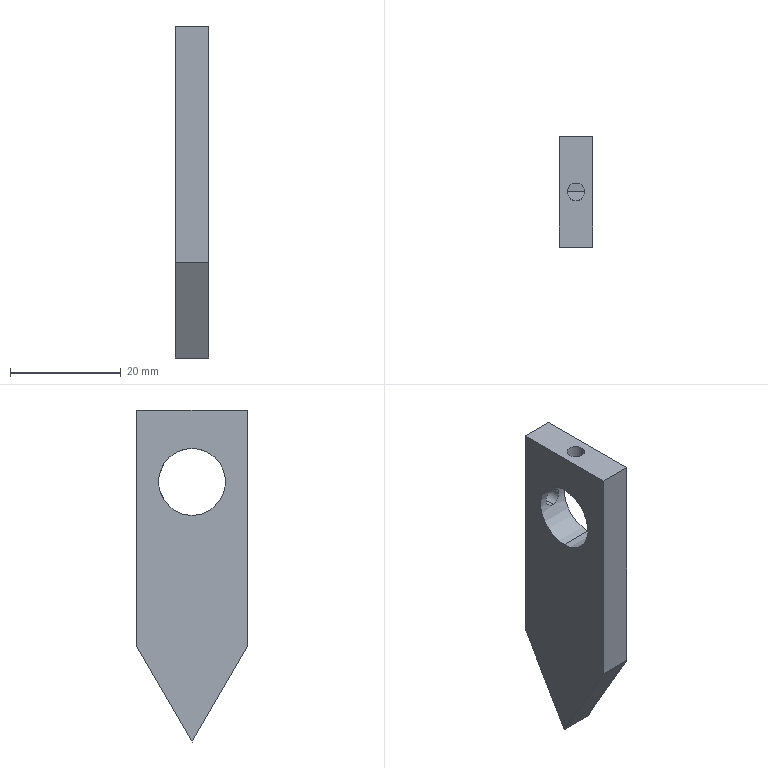Part | STEP file | 1 solid | 13 faces | box 6 x 20 x 60 mm | volume 5382 mm3 | plane 7 | cylinder 6 | commonest cylinder face diameters 3.2 x4 12.1 x2